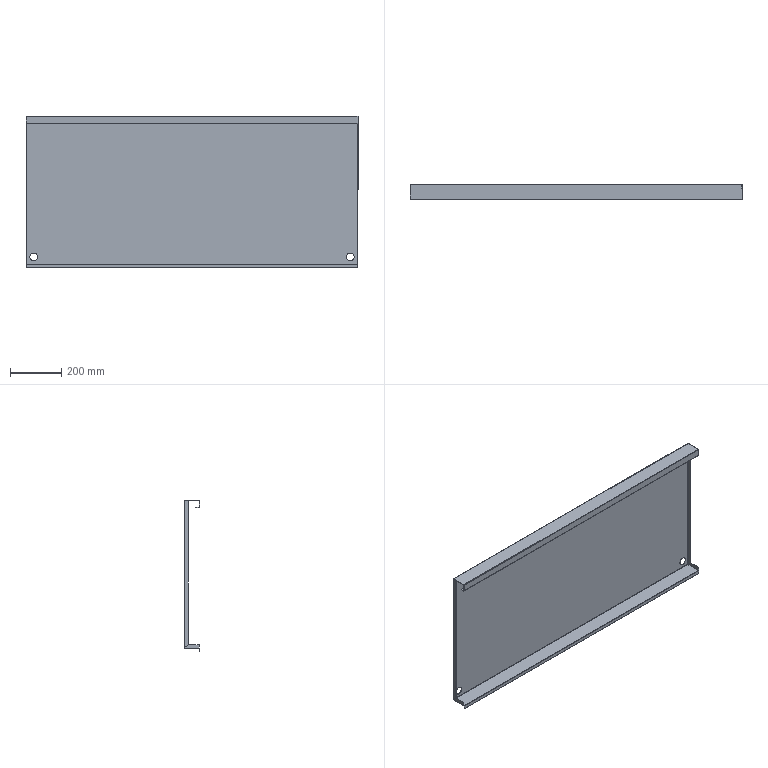Part | SolidWorks | features EdgeFlange 3, FlatPattern 1, ICE 1, SMBaseFlange 1, SheetMetal 1 | 1 solid | 88 faces | box 1298 x 60 x 593.8 mm | volume 1188621 mm3 | plane 62 | cylinder 22 | spline 4 | commonest cylinder face diameters 0.9 x9 3.3 x9 30 x4